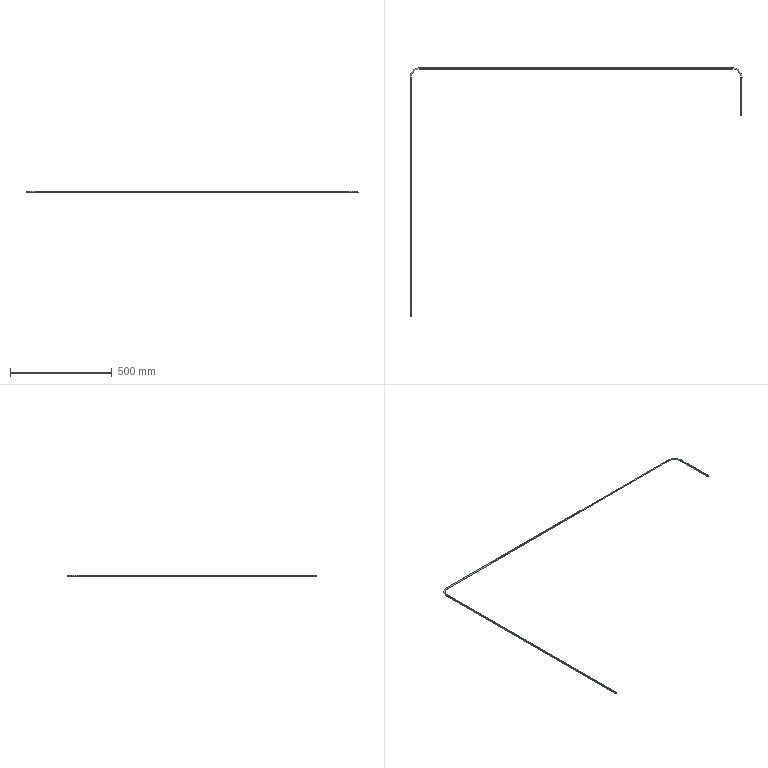Part | SolidWorks | features Sweep 1 | 1 solid | 12 faces | box 1629 x 1218 x 6.5 mm | volume 100576 mm3 | cylinder 6 | torus 4 | plane 2 | commonest cylinder face diameters 6.5 x6
STEP:
#1=CARTESIAN_POINT('',(1580.,1215.,-3.25));
#2=VERTEX_POINT('',#1);
#3=CARTESIAN_POINT('',(1580.,1218.25,0.));
#4=VERTEX_POINT('',#3);
#5=CARTESIAN_POINT('',(1580.,1215.,0.));
#6=DIRECTION('',(1.,0.,0.));
#7=DIRECTION('',(0.,0.,1.));
#8=AXIS2_PLACEMENT_3D('',#5,#6,#7);
#9=CIRCLE('',#8,3.25);
#10=EDGE_CURVE('',#2,#4,#9,.T.);
#11=ORIENTED_EDGE('',*,*,#10,.T.);
#12=CARTESIAN_POINT('',(1625.25,1173.,0.));
#13=VERTEX_POINT('',#12);
#14=CARTESIAN_POINT('',(1580.,1173.,0.));
#15=DIRECTION('',(0.,0.,-1.));
#16=DIRECTION('',(-1.,0.,0.));
#17=AXIS2_PLACEMENT_3D('',#14,#15,#16);
#18=CIRCLE('',#17,45.25);
#19=EDGE_CURVE('',#4,#13,#18,.T.);
#20=ORIENTED_EDGE('',*,*,#19,.T.);
#21=CARTESIAN_POINT('',(1622.,1173.,-3.25));
#22=VERTEX_POINT('',#21);
#23=CARTESIAN_POINT('',(1622.,1173.,0.));
#24=DIRECTION('',(0.,-1.,0.));
#25=DIRECTION('',(0.,0.,1.));
#26=AXIS2_PLACEMENT_3D('',#23,#24,#25);
#27=CIRCLE('',#26,3.25);
#28=EDGE_CURVE('',#22,#13,#27,.T.);
#29=ORIENTED_EDGE('',*,*,#28,.F.);
#30=CARTESIAN_POINT('',(1618.75,1173.,0.));
#31=VERTEX_POINT('',#30);
#32=CARTESIAN_POINT('',(1622.,1173.,0.));
#33=DIRECTION('',(0.,-1.,0.));
#34=DIRECTION('',(0.,0.,1.));
#35=AXIS2_PLACEMENT_3D('',#32,#33,#34);
#36=CIRCLE('',#35,3.25);
#37=EDGE_CURVE('',#31,#22,#36,.T.);
#38=ORIENTED_EDGE('',*,*,#37,.F.);
#39=CARTESIAN_POINT('',(1580.,1211.75,0.));
#40=VERTEX_POINT('',#39);
#41=CARTESIAN_POINT('',(1580.,1173.,0.));
#42=DIRECTION('',(0.,0.,-1.));
#43=DIRECTION('',(-1.,0.,0.));
#44=AXIS2_PLACEMENT_3D('',#41,#42,#43);
#45=CIRCLE('',#44,38.75);
#46=EDGE_CURVE('',#40,#31,#45,.T.);
#47=ORIENTED_EDGE('',*,*,#46,.F.);
#48=CARTESIAN_POINT('',(1580.,1215.,0.));
#49=DIRECTION('',(1.,0.,0.));
#50=DIRECTION('',(0.,0.,1.));
#51=AXIS2_PLACEMENT_3D('',#48,#49,#50);
#52=CIRCLE('',#51,3.25);
#53=EDGE_CURVE('',#40,#2,#52,.T.);
#54=ORIENTED_EDGE('',*,*,#53,.T.);
#55=EDGE_LOOP('',(#11,#20,#29,#38,#47,#54));
#56=FACE_OUTER_BOUND('',#55,.T.);
#57=CARTESIAN_POINT('',(1580.,1173.,0.));
#58=DIRECTION('',(0.,0.,-1.));
#59=DIRECTION('',(-1.,0.,0.));
#60=AXIS2_PLACEMENT_3D('',#57,#58,#59);
#61=TOROIDAL_SURFACE('',#60,42.,3.25);
#62=ADVANCED_FACE('',(#56),#61,.T.);
#63=CARTESIAN_POINT('',(0.,1173.,-3.25));
#64=VERTEX_POINT('',#63);
#65=CARTESIAN_POINT('',(-3.25,1173.,0.));
#66=VERTEX_POINT('',#65);
#67=CARTESIAN_POINT('',(0.,1173.,0.));
#68=DIRECTION('',(0.,1.,0.));
#69=DIRECTION('',(0.,0.,1.));
#70=AXIS2_PLACEMENT_3D('',#67,#68,#69);
#71=CIRCLE('',#70,3.25);
#72=EDGE_CURVE('',#64,#66,#71,.T.);
#73=ORIENTED_EDGE('',*,*,#72,.T.);
#74=CARTESIAN_POINT('',(42.,1218.25,0.));
#75=VERTEX_POINT('',#74);
#76=CARTESIAN_POINT('',(42.,1173.,0.));
#77=DIRECTION('',(0.,0.,-1.));
#78=DIRECTION('',(-1.,0.,0.));
#79=AXIS2_PLACEMENT_3D('',#76,#77,#78);
#80=CIRCLE('',#79,45.25);
#81=EDGE_CURVE('',#66,#75,#80,.T.);
#82=ORIENTED_EDGE('',*,*,#81,.T.);
#83=CARTESIAN_POINT('',(42.,1215.,-3.25));
#84=VERTEX_POINT('',#83);
#85=CARTESIAN_POINT('',(42.,1215.,0.));
#86=DIRECTION('',(1.,0.,0.));
#87=DIRECTION('',(0.,0.,1.));
#88=AXIS2_PLACEMENT_3D('',#85,#86,#87);
#89=CIRCLE('',#88,3.25);
#90=EDGE_CURVE('',#84,#75,#89,.T.);
#91=ORIENTED_EDGE('',*,*,#90,.F.);
#92=CARTESIAN_POINT('',(42.,1211.75,0.));
#93=VERTEX_POINT('',#92);
#94=CARTESIAN_POINT('',(42.,1215.,0.));
#95=DIRECTION('',(1.,0.,0.));
#96=DIRECTION('',(0.,0.,1.));
#97=AXIS2_PLACEMENT_3D('',#94,#95,#96);
#98=CIRCLE('',#97,3.25);
#99=EDGE_CURVE('',#93,#84,#98,.T.);
#100=ORIENTED_EDGE('',*,*,#99,.F.);
#101=CARTESIAN_POINT('',(3.25,1173.,0.));
#102=VERTEX_POINT('',#101);
#103=CARTESIAN_POINT('',(42.,1173.,0.));
#104=DIRECTION('',(0.,0.,-1.));
#105=DIRECTION('',(-1.,0.,0.));
#106=AXIS2_PLACEMENT_3D('',#103,#104,#105);
#107=CIRCLE('',#106,38.75);
#108=EDGE_CURVE('',#102,#93,#107,.T.);
#109=ORIENTED_EDGE('',*,*,#108,.F.);
#110=CARTESIAN_POINT('',(0.,1173.,0.));
#111=DIRECTION('',(0.,1.,0.));
#112=DIRECTION('',(0.,0.,1.));
#113=AXIS2_PLACEMENT_3D('',#110,#111,#112);
#114=CIRCLE('',#113,3.25);
#115=EDGE_CURVE('',#102,#64,#114,.T.);
#116=ORIENTED_EDGE('',*,*,#115,.T.);
#117=EDGE_LOOP('',(#73,#82,#91,#100,#109,#116));
#118=FACE_OUTER_BOUND('',#117,.T.);
#119=CARTESIAN_POINT('',(42.,1173.,0.));
#120=DIRECTION('',(0.,0.,-1.));
#121=DIRECTION('',(-1.,0.,0.));
#122=AXIS2_PLACEMENT_3D('',#119,#120,#121);
#123=TOROIDAL_SURFACE('',#122,42.,3.25);
#124=ADVANCED_FACE('',(#118),#123,.T.);
#125=ORIENTED_EDGE('',*,*,#28,.T.);
#126=CARTESIAN_POINT('',(1622.,1173.,3.25));
#127=VERTEX_POINT('',#126);
#128=CARTESIAN_POINT('',(1622.,1173.,0.));
#129=DIRECTION('',(0.,-1.,0.));
#130=DIRECTION('',(0.,0.,1.));
#131=AXIS2_PLACEMENT_3D('',#128,#129,#130);
#132=CIRCLE('',#131,3.25);
#133=EDGE_CURVE('',#13,#127,#132,.T.);
#134=ORIENTED_EDGE('',*,*,#133,.T.);
#135=CARTESIAN_POINT('',(1622.,985.,3.25));
#136=VERTEX_POINT('',#135);
#137=CARTESIAN_POINT('',(1622.,1173.,3.25));
#138=DIRECTION('',(0.,-1.,0.));
#139=VECTOR('',#138,1000.);
#140=LINE('',#137,#139);
#141=EDGE_CURVE('',#127,#136,#140,.T.);
#142=ORIENTED_EDGE('',*,*,#141,.T.);
#143=CARTESIAN_POINT('',(1622.,985.,-3.25));
#144=VERTEX_POINT('',#143);
#145=CARTESIAN_POINT('',(1622.,985.,0.));
#146=DIRECTION('',(0.,-1.,0.));
#147=DIRECTION('',(0.,0.,1.));
#148=AXIS2_PLACEMENT_3D('',#145,#146,#147);
#149=CIRCLE('',#148,3.25);
#150=EDGE_CURVE('',#144,#136,#149,.T.);
#151=ORIENTED_EDGE('',*,*,#150,.F.);
#152=CARTESIAN_POINT('',(1622.,1173.,-3.25));
#153=DIRECTION('',(0.,-1.,0.));
#154=VECTOR('',#153,1000.);
#155=LINE('',#152,#154);
#156=EDGE_CURVE('',#22,#144,#155,.T.);
#157=ORIENTED_EDGE('',*,*,#156,.F.);
#158=EDGE_LOOP('',(#125,#134,#142,#151,#157));
#159=FACE_OUTER_BOUND('',#158,.T.);
#160=CARTESIAN_POINT('',(1622.,1173.,0.));
#161=DIRECTION('',(0.,-1.,0.));
#162=DIRECTION('',(0.,0.,-1.));
#163=AXIS2_PLACEMENT_3D('',#160,#161,#162);
#164=CYLINDRICAL_SURFACE('',#163,3.25);
#165=ADVANCED_FACE('',(#159),#164,.T.);
#166=ORIENTED_EDGE('',*,*,#90,.T.);
#167=CARTESIAN_POINT('',(42.,1215.,3.25));
#168=VERTEX_POINT('',#167);
#169=CARTESIAN_POINT('',(42.,1215.,0.));
#170=DIRECTION('',(1.,0.,0.));
#171=DIRECTION('',(0.,0.,1.));
#172=AXIS2_PLACEMENT_3D('',#169,#170,#171);
#173=CIRCLE('',#172,3.25);
#174=EDGE_CURVE('',#75,#168,#173,.T.);
#175=ORIENTED_EDGE('',*,*,#174,.T.);
#176=CARTESIAN_POINT('',(1580.,1215.,3.25));
#177=VERTEX_POINT('',#176);
#178=CARTESIAN_POINT('',(42.,1215.,3.25));
#179=DIRECTION('',(1.,0.,0.));
#180=VECTOR('',#179,1000.);
#181=LINE('',#178,#180);
#182=EDGE_CURVE('',#168,#177,#181,.T.);
#183=ORIENTED_EDGE('',*,*,#182,.T.);
#184=CARTESIAN_POINT('',(1580.,1215.,0.));
#185=DIRECTION('',(1.,0.,0.));
#186=DIRECTION('',(0.,0.,1.));
#187=AXIS2_PLACEMENT_3D('',#184,#185,#186);
#188=CIRCLE('',#187,3.25);
#189=EDGE_CURVE('',#4,#177,#188,.T.);
#190=ORIENTED_EDGE('',*,*,#189,.F.);
#191=ORIENTED_EDGE('',*,*,#10,.F.);
#192=CARTESIAN_POINT('',(42.,1215.,-3.25));
#193=DIRECTION('',(1.,0.,0.));
#194=VECTOR('',#193,1000.);
#195=LINE('',#192,#194);
#196=EDGE_CURVE('',#84,#2,#195,.T.);
#197=ORIENTED_EDGE('',*,*,#196,.F.);
#198=EDGE_LOOP('',(#166,#175,#183,#190,#191,#197));
#199=FACE_OUTER_BOUND('',#198,.T.);
#200=CARTESIAN_POINT('',(42.,1215.,0.));
#201=DIRECTION('',(1.,0.,0.));
#202=DIRECTION('',(0.,0.,-1.));
#203=AXIS2_PLACEMENT_3D('',#200,#201,#202);
#204=CYLINDRICAL_SURFACE('',#203,3.25);
#205=ADVANCED_FACE('',(#199),#204,.T.);
#206=CARTESIAN_POINT('',(0.,0.,3.25));
#207=VERTEX_POINT('',#206);
#208=CARTESIAN_POINT('',(0.,0.,-3.25));
#209=VERTEX_POINT('',#208);
#210=CARTESIAN_POINT('',(0.,0.,0.));
#211=DIRECTION('',(0.,1.,0.));
#212=DIRECTION('',(0.,0.,1.));
#213=AXIS2_PLACEMENT_3D('',#210,#211,#212);
#214=CIRCLE('',#213,3.25);
#215=EDGE_CURVE('',#207,#209,#214,.T.);
#216=ORIENTED_EDGE('',*,*,#215,.T.);
#217=CARTESIAN_POINT('',(0.,0.,-3.25));
#218=DIRECTION('',(0.,1.,0.));
#219=VECTOR('',#218,1000.);
#220=LINE('',#217,#219);
#221=EDGE_CURVE('',#209,#64,#220,.T.);
#222=ORIENTED_EDGE('',*,*,#221,.T.);
#223=ORIENTED_EDGE('',*,*,#115,.F.);
#224=CARTESIAN_POINT('',(0.,1173.,3.25));
#225=VERTEX_POINT('',#224);
#226=CARTESIAN_POINT('',(0.,1173.,0.));
#227=DIRECTION('',(0.,1.,0.));
#228=DIRECTION('',(0.,0.,1.));
#229=AXIS2_PLACEMENT_3D('',#226,#227,#228);
#230=CIRCLE('',#229,3.25);
#231=EDGE_CURVE('',#225,#102,#230,.T.);
#232=ORIENTED_EDGE('',*,*,#231,.F.);
#233=CARTESIAN_POINT('',(0.,0.,3.25));
#234=DIRECTION('',(0.,1.,0.));
#235=VECTOR('',#234,1000.);
#236=LINE('',#233,#235);
#237=EDGE_CURVE('',#207,#225,#236,.T.);
#238=ORIENTED_EDGE('',*,*,#237,.F.);
#239=EDGE_LOOP('',(#216,#222,#223,#232,#238));
#240=FACE_OUTER_BOUND('',#239,.T.);
#241=CARTESIAN_POINT('',(0.,0.,0.));
#242=DIRECTION('',(0.,1.,0.));
#243=DIRECTION('',(0.,0.,1.));
#244=AXIS2_PLACEMENT_3D('',#241,#242,#243);
#245=CYLINDRICAL_SURFACE('',#244,3.25);
#246=ADVANCED_FACE('',(#240),#245,.T.);
#247=ORIENTED_EDGE('',*,*,#141,.F.);
#248=CARTESIAN_POINT('',(1622.,1173.,0.));
#249=DIRECTION('',(0.,-1.,0.));
#250=DIRECTION('',(0.,0.,1.));
#251=AXIS2_PLACEMENT_3D('',#248,#249,#250);
#252=CIRCLE('',#251,3.25);
#253=EDGE_CURVE('',#127,#31,#252,.T.);
#254=ORIENTED_EDGE('',*,*,#253,.T.);
#255=ORIENTED_EDGE('',*,*,#37,.T.);
#256=ORIENTED_EDGE('',*,*,#156,.T.);
#257=CARTESIAN_POINT('',(1622.,985.,0.));
#258=DIRECTION('',(0.,-1.,0.));
#259=DIRECTION('',(0.,0.,1.));
#260=AXIS2_PLACEMENT_3D('',#257,#258,#259);
#261=CIRCLE('',#260,3.25);
#262=EDGE_CURVE('',#136,#144,#261,.T.);
#263=ORIENTED_EDGE('',*,*,#262,.F.);
#264=EDGE_LOOP('',(#247,#254,#255,#256,#263));
#265=FACE_OUTER_BOUND('',#264,.T.);
#266=CARTESIAN_POINT('',(1622.,1173.,0.));
#267=DIRECTION('',(0.,-1.,0.));
#268=DIRECTION('',(0.,0.,-1.));
#269=AXIS2_PLACEMENT_3D('',#266,#267,#268);
#270=CYLINDRICAL_SURFACE('',#269,3.25);
#271=ADVANCED_FACE('',(#265),#270,.T.);
#272=ORIENTED_EDGE('',*,*,#19,.F.);
#273=ORIENTED_EDGE('',*,*,#189,.T.);
#274=CARTESIAN_POINT('',(1580.,1215.,0.));
#275=DIRECTION('',(1.,0.,0.));
#276=DIRECTION('',(0.,0.,1.));
#277=AXIS2_PLACEMENT_3D('',#274,#275,#276);
#278=CIRCLE('',#277,3.25);
#279=EDGE_CURVE('',#177,#40,#278,.T.);
#280=ORIENTED_EDGE('',*,*,#279,.T.);
#281=ORIENTED_EDGE('',*,*,#46,.T.);
#282=ORIENTED_EDGE('',*,*,#253,.F.);
#283=ORIENTED_EDGE('',*,*,#133,.F.);
#284=EDGE_LOOP('',(#272,#273,#280,#281,#282,#283));
#285=FACE_OUTER_BOUND('',#284,.T.);
#286=CARTESIAN_POINT('',(1580.,1173.,0.));
#287=DIRECTION('',(0.,0.,-1.));
#288=DIRECTION('',(-1.,0.,0.));
#289=AXIS2_PLACEMENT_3D('',#286,#287,#288);
#290=TOROIDAL_SURFACE('',#289,42.,3.25);
#291=ADVANCED_FACE('',(#285),#290,.T.);
#292=ORIENTED_EDGE('',*,*,#182,.F.);
#293=CARTESIAN_POINT('',(42.,1215.,0.));
#294=DIRECTION('',(1.,0.,0.));
#295=DIRECTION('',(0.,0.,1.));
#296=AXIS2_PLACEMENT_3D('',#293,#294,#295);
#297=CIRCLE('',#296,3.25);
#298=EDGE_CURVE('',#168,#93,#297,.T.);
#299=ORIENTED_EDGE('',*,*,#298,.T.);
#300=ORIENTED_EDGE('',*,*,#99,.T.);
#301=ORIENTED_EDGE('',*,*,#196,.T.);
#302=ORIENTED_EDGE('',*,*,#53,.F.);
#303=ORIENTED_EDGE('',*,*,#279,.F.);
#304=EDGE_LOOP('',(#292,#299,#300,#301,#302,#303));
#305=FACE_OUTER_BOUND('',#304,.T.);
#306=CARTESIAN_POINT('',(42.,1215.,0.));
#307=DIRECTION('',(1.,0.,0.));
#308=DIRECTION('',(0.,0.,-1.));
#309=AXIS2_PLACEMENT_3D('',#306,#307,#308);
#310=CYLINDRICAL_SURFACE('',#309,3.25);
#311=ADVANCED_FACE('',(#305),#310,.T.);
#312=ORIENTED_EDGE('',*,*,#81,.F.);
#313=CARTESIAN_POINT('',(0.,1173.,0.));
#314=DIRECTION('',(0.,1.,0.));
#315=DIRECTION('',(0.,0.,1.));
#316=AXIS2_PLACEMENT_3D('',#313,#314,#315);
#317=CIRCLE('',#316,3.25);
#318=EDGE_CURVE('',#66,#225,#317,.T.);
#319=ORIENTED_EDGE('',*,*,#318,.T.);
#320=ORIENTED_EDGE('',*,*,#231,.T.);
#321=ORIENTED_EDGE('',*,*,#108,.T.);
#322=ORIENTED_EDGE('',*,*,#298,.F.);
#323=ORIENTED_EDGE('',*,*,#174,.F.);
#324=EDGE_LOOP('',(#312,#319,#320,#321,#322,#323));
#325=FACE_OUTER_BOUND('',#324,.T.);
#326=CARTESIAN_POINT('',(42.,1173.,0.));
#327=DIRECTION('',(0.,0.,-1.));
#328=DIRECTION('',(-1.,0.,0.));
#329=AXIS2_PLACEMENT_3D('',#326,#327,#328);
#330=TOROIDAL_SURFACE('',#329,42.,3.25);
#331=ADVANCED_FACE('',(#325),#330,.T.);
#332=ORIENTED_EDGE('',*,*,#221,.F.);
#333=CARTESIAN_POINT('',(0.,0.,0.));
#334=DIRECTION('',(0.,1.,0.));
#335=DIRECTION('',(0.,0.,1.));
#336=AXIS2_PLACEMENT_3D('',#333,#334,#335);
#337=CIRCLE('',#336,3.25);
#338=EDGE_CURVE('',#209,#207,#337,.T.);
#339=ORIENTED_EDGE('',*,*,#338,.T.);
#340=ORIENTED_EDGE('',*,*,#237,.T.);
#341=ORIENTED_EDGE('',*,*,#318,.F.);
#342=ORIENTED_EDGE('',*,*,#72,.F.);
#343=EDGE_LOOP('',(#332,#339,#340,#341,#342));
#344=FACE_OUTER_BOUND('',#343,.T.);
#345=CARTESIAN_POINT('',(0.,0.,0.));
#346=DIRECTION('',(0.,1.,0.));
#347=DIRECTION('',(0.,0.,1.));
#348=AXIS2_PLACEMENT_3D('',#345,#346,#347);
#349=CYLINDRICAL_SURFACE('',#348,3.25);
#350=ADVANCED_FACE('',(#344),#349,.T.);
#351=ORIENTED_EDGE('',*,*,#150,.T.);
#352=ORIENTED_EDGE('',*,*,#262,.T.);
#353=EDGE_LOOP('',(#351,#352));
#354=FACE_OUTER_BOUND('',#353,.T.);
#355=CARTESIAN_POINT('',(1622.,985.,0.));
#356=DIRECTION('',(0.,-1.,0.));
#357=DIRECTION('',(0.,0.,1.));
#358=AXIS2_PLACEMENT_3D('',#355,#356,#357);
#359=PLANE('',#358);
#360=ADVANCED_FACE('',(#354),#359,.T.);
#361=ORIENTED_EDGE('',*,*,#215,.F.);
#362=ORIENTED_EDGE('',*,*,#338,.F.);
#363=EDGE_LOOP('',(#361,#362));
#364=FACE_OUTER_BOUND('',#363,.T.);
#365=CARTESIAN_POINT('',(0.,0.,0.));
#366=DIRECTION('',(0.,1.,0.));
#367=DIRECTION('',(0.,0.,1.));
#368=AXIS2_PLACEMENT_3D('',#365,#366,#367);
#369=PLANE('',#368);
#370=ADVANCED_FACE('',(#364),#369,.F.);
#371=CLOSED_SHELL('',(#62,#124,#165,#205,#246,#271,#291,#311,#331,#350,#360,#370));
#372=MANIFOLD_SOLID_BREP('',#371);
#373=CARTESIAN_POINT('',(0.,0.,0.));
#374=DIRECTION('',(0.,0.,1.));
#375=DIRECTION('',(1.,0.,0.));
#376=AXIS2_PLACEMENT_3D('',#373,#374,#375);
#377=(LENGTH_UNIT()NAMED_UNIT(*)SI_UNIT(.MILLI.,.METRE.));
#378=UNCERTAINTY_MEASURE_WITH_UNIT(LENGTH_MEASURE(0.00001),#377,'','');
#379=(NAMED_UNIT(*)PLANE_ANGLE_UNIT()SI_UNIT($,.RADIAN.));
#380=(NAMED_UNIT(*)SI_UNIT($,.STERADIAN.)SOLID_ANGLE_UNIT());
#381=(GEOMETRIC_REPRESENTATION_CONTEXT(3)GLOBAL_UNCERTAINTY_ASSIGNED_CONTEXT((#378))GLOBAL_UNIT_ASSIGNED_CONTEXT((#377,#379,#380))REPRESENTATION_CONTEXT('',''));
#382=ADVANCED_BREP_SHAPE_REPRESENTATION('',(#372,#376),#381);